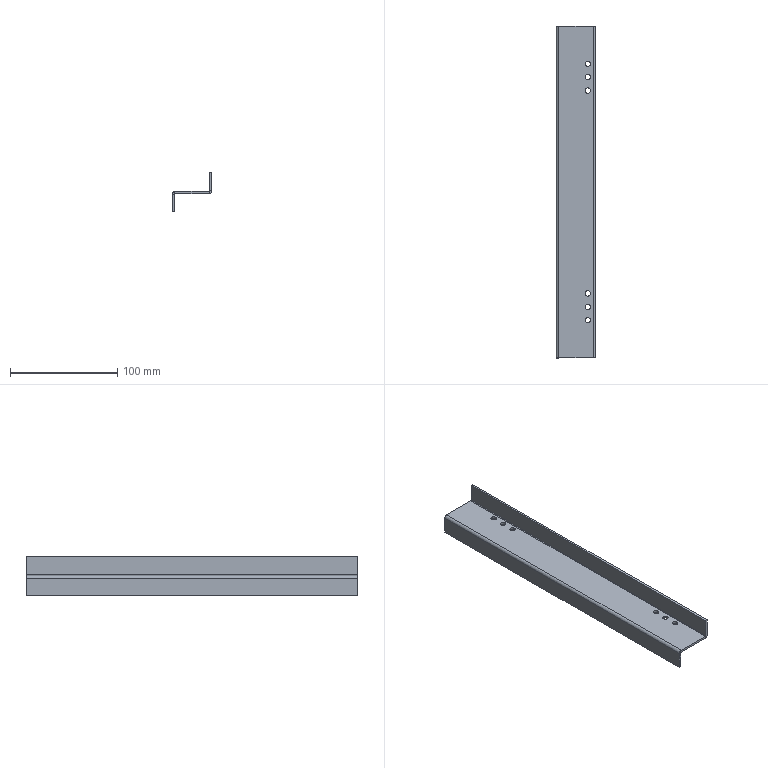Part | SolidWorks | features BaseBody 1 | 1 solid | 34 faces | box 37 x 310 x 36 mm | volume 42986 mm3 | plane 18 | cylinder 16 | commonest cylinder face diameters 5 x14 1 x2
STEP:
#1=CARTESIAN_POINT('',(13.5,119.75,0.));
#2=VERTEX_POINT('',#1);
#3=CARTESIAN_POINT('',(13.5,119.75,-2.));
#4=VERTEX_POINT('',#3);
#5=CARTESIAN_POINT('',(13.5,119.75,0.));
#6=DIRECTION('',(0.,0.,-1.));
#7=VECTOR('',#6,1000.);
#8=LINE('',#5,#7);
#9=EDGE_CURVE('',#2,#4,#8,.T.);
#10=ORIENTED_EDGE('',*,*,#9,.F.);
#11=CARTESIAN_POINT('',(8.5,119.75,0.));
#12=VERTEX_POINT('',#11);
#13=CARTESIAN_POINT('',(11.,119.75,0.));
#14=DIRECTION('',(0.,0.,-1.));
#15=DIRECTION('',(-1.,0.,0.));
#16=AXIS2_PLACEMENT_3D('',#13,#14,#15);
#17=CIRCLE('',#16,2.5);
#18=EDGE_CURVE('',#12,#2,#17,.T.);
#19=ORIENTED_EDGE('',*,*,#18,.F.);
#20=CARTESIAN_POINT('',(8.5,119.75,-2.));
#21=VERTEX_POINT('',#20);
#22=CARTESIAN_POINT('',(8.5,119.75,0.));
#23=DIRECTION('',(0.,0.,-1.));
#24=VECTOR('',#23,1000.);
#25=LINE('',#22,#24);
#26=EDGE_CURVE('',#12,#21,#25,.T.);
#27=ORIENTED_EDGE('',*,*,#26,.T.);
#28=CARTESIAN_POINT('',(11.,119.75,-2.));
#29=DIRECTION('',(0.,0.,-1.));
#30=DIRECTION('',(-1.,0.,0.));
#31=AXIS2_PLACEMENT_3D('',#28,#29,#30);
#32=CIRCLE('',#31,2.5);
#33=EDGE_CURVE('',#21,#4,#32,.T.);
#34=ORIENTED_EDGE('',*,*,#33,.T.);
#35=EDGE_LOOP('',(#10,#19,#27,#34));
#36=FACE_OUTER_BOUND('',#35,.T.);
#37=CARTESIAN_POINT('',(11.,119.75,0.));
#38=DIRECTION('',(0.,0.,-1.));
#39=DIRECTION('',(-1.,0.,0.));
#40=AXIS2_PLACEMENT_3D('',#37,#38,#39);
#41=CYLINDRICAL_SURFACE('',#40,2.5);
#42=ADVANCED_FACE('',(#36),#41,.F.);
#43=CARTESIAN_POINT('',(13.5,94.75,0.));
#44=VERTEX_POINT('',#43);
#45=CARTESIAN_POINT('',(13.5,94.75,-2.));
#46=VERTEX_POINT('',#45);
#47=CARTESIAN_POINT('',(13.5,94.75,0.));
#48=DIRECTION('',(0.,0.,-1.));
#49=VECTOR('',#48,1000.);
#50=LINE('',#47,#49);
#51=EDGE_CURVE('',#44,#46,#50,.T.);
#52=ORIENTED_EDGE('',*,*,#51,.F.);
#53=CARTESIAN_POINT('',(8.5,94.75,0.));
#54=VERTEX_POINT('',#53);
#55=CARTESIAN_POINT('',(11.,94.75,0.));
#56=DIRECTION('',(0.,0.,-1.));
#57=DIRECTION('',(-1.,0.,0.));
#58=AXIS2_PLACEMENT_3D('',#55,#56,#57);
#59=CIRCLE('',#58,2.5);
#60=EDGE_CURVE('',#54,#44,#59,.T.);
#61=ORIENTED_EDGE('',*,*,#60,.F.);
#62=CARTESIAN_POINT('',(8.5,94.75,-2.));
#63=VERTEX_POINT('',#62);
#64=CARTESIAN_POINT('',(8.5,94.75,0.));
#65=DIRECTION('',(0.,0.,-1.));
#66=VECTOR('',#65,1000.);
#67=LINE('',#64,#66);
#68=EDGE_CURVE('',#54,#63,#67,.T.);
#69=ORIENTED_EDGE('',*,*,#68,.T.);
#70=CARTESIAN_POINT('',(11.,94.75,-2.));
#71=DIRECTION('',(0.,0.,-1.));
#72=DIRECTION('',(-1.,0.,0.));
#73=AXIS2_PLACEMENT_3D('',#70,#71,#72);
#74=CIRCLE('',#73,2.5);
#75=EDGE_CURVE('',#63,#46,#74,.T.);
#76=ORIENTED_EDGE('',*,*,#75,.T.);
#77=EDGE_LOOP('',(#52,#61,#69,#76));
#78=FACE_OUTER_BOUND('',#77,.T.);
#79=CARTESIAN_POINT('',(11.,94.75,0.));
#80=DIRECTION('',(0.,0.,-1.));
#81=DIRECTION('',(-1.,0.,0.));
#82=AXIS2_PLACEMENT_3D('',#79,#80,#81);
#83=CYLINDRICAL_SURFACE('',#82,2.5);
#84=ADVANCED_FACE('',(#78),#83,.F.);
#85=CARTESIAN_POINT('',(13.5,-119.75,0.));
#86=VERTEX_POINT('',#85);
#87=CARTESIAN_POINT('',(13.5,-119.75,-2.));
#88=VERTEX_POINT('',#87);
#89=CARTESIAN_POINT('',(13.5,-119.75,0.));
#90=DIRECTION('',(0.,0.,-1.));
#91=VECTOR('',#90,1000.);
#92=LINE('',#89,#91);
#93=EDGE_CURVE('',#86,#88,#92,.T.);
#94=ORIENTED_EDGE('',*,*,#93,.F.);
#95=CARTESIAN_POINT('',(8.5,-119.75,0.));
#96=VERTEX_POINT('',#95);
#97=CARTESIAN_POINT('',(11.,-119.75,0.));
#98=DIRECTION('',(0.,0.,-1.));
#99=DIRECTION('',(1.,0.,0.));
#100=AXIS2_PLACEMENT_3D('',#97,#98,#99);
#101=CIRCLE('',#100,2.5);
#102=EDGE_CURVE('',#96,#86,#101,.T.);
#103=ORIENTED_EDGE('',*,*,#102,.F.);
#104=CARTESIAN_POINT('',(8.5,-119.75,-2.));
#105=VERTEX_POINT('',#104);
#106=CARTESIAN_POINT('',(8.5,-119.75,0.));
#107=DIRECTION('',(0.,0.,-1.));
#108=VECTOR('',#107,1000.);
#109=LINE('',#106,#108);
#110=EDGE_CURVE('',#96,#105,#109,.T.);
#111=ORIENTED_EDGE('',*,*,#110,.T.);
#112=CARTESIAN_POINT('',(11.,-119.75,-2.));
#113=DIRECTION('',(0.,0.,-1.));
#114=DIRECTION('',(1.,0.,0.));
#115=AXIS2_PLACEMENT_3D('',#112,#113,#114);
#116=CIRCLE('',#115,2.5);
#117=EDGE_CURVE('',#105,#88,#116,.T.);
#118=ORIENTED_EDGE('',*,*,#117,.T.);
#119=EDGE_LOOP('',(#94,#103,#111,#118));
#120=FACE_OUTER_BOUND('',#119,.T.);
#121=CARTESIAN_POINT('',(11.,-119.75,0.));
#122=DIRECTION('',(0.,0.,-1.));
#123=DIRECTION('',(-1.,0.,0.));
#124=AXIS2_PLACEMENT_3D('',#121,#122,#123);
#125=CYLINDRICAL_SURFACE('',#124,2.5);
#126=ADVANCED_FACE('',(#120),#125,.F.);
#127=CARTESIAN_POINT('',(13.5,-94.75,0.));
#128=VERTEX_POINT('',#127);
#129=CARTESIAN_POINT('',(13.5,-94.75,-2.));
#130=VERTEX_POINT('',#129);
#131=CARTESIAN_POINT('',(13.5,-94.75,0.));
#132=DIRECTION('',(0.,0.,-1.));
#133=VECTOR('',#132,1000.);
#134=LINE('',#131,#133);
#135=EDGE_CURVE('',#128,#130,#134,.T.);
#136=ORIENTED_EDGE('',*,*,#135,.F.);
#137=CARTESIAN_POINT('',(8.5,-94.75,0.));
#138=VERTEX_POINT('',#137);
#139=CARTESIAN_POINT('',(11.,-94.75,0.));
#140=DIRECTION('',(0.,0.,-1.));
#141=DIRECTION('',(1.,0.,0.));
#142=AXIS2_PLACEMENT_3D('',#139,#140,#141);
#143=CIRCLE('',#142,2.5);
#144=EDGE_CURVE('',#138,#128,#143,.T.);
#145=ORIENTED_EDGE('',*,*,#144,.F.);
#146=CARTESIAN_POINT('',(8.5,-94.75,-2.));
#147=VERTEX_POINT('',#146);
#148=CARTESIAN_POINT('',(8.5,-94.75,0.));
#149=DIRECTION('',(0.,0.,-1.));
#150=VECTOR('',#149,1000.);
#151=LINE('',#148,#150);
#152=EDGE_CURVE('',#138,#147,#151,.T.);
#153=ORIENTED_EDGE('',*,*,#152,.T.);
#154=CARTESIAN_POINT('',(11.,-94.75,-2.));
#155=DIRECTION('',(0.,0.,-1.));
#156=DIRECTION('',(1.,0.,0.));
#157=AXIS2_PLACEMENT_3D('',#154,#155,#156);
#158=CIRCLE('',#157,2.5);
#159=EDGE_CURVE('',#147,#130,#158,.T.);
#160=ORIENTED_EDGE('',*,*,#159,.T.);
#161=EDGE_LOOP('',(#136,#145,#153,#160));
#162=FACE_OUTER_BOUND('',#161,.T.);
#163=CARTESIAN_POINT('',(11.,-94.75,0.));
#164=DIRECTION('',(0.,0.,-1.));
#165=DIRECTION('',(-1.,0.,0.));
#166=AXIS2_PLACEMENT_3D('',#163,#164,#165);
#167=CYLINDRICAL_SURFACE('',#166,2.5);
#168=ADVANCED_FACE('',(#162),#167,.F.);
#169=CARTESIAN_POINT('',(13.5,-107.25,0.));
#170=VERTEX_POINT('',#169);
#171=CARTESIAN_POINT('',(13.5,-107.25,-2.));
#172=VERTEX_POINT('',#171);
#173=CARTESIAN_POINT('',(13.5,-107.25,0.));
#174=DIRECTION('',(0.,0.,-1.));
#175=VECTOR('',#174,1000.);
#176=LINE('',#173,#175);
#177=EDGE_CURVE('',#170,#172,#176,.T.);
#178=ORIENTED_EDGE('',*,*,#177,.F.);
#179=CARTESIAN_POINT('',(8.5,-107.25,0.));
#180=VERTEX_POINT('',#179);
#181=CARTESIAN_POINT('',(11.,-107.25,0.));
#182=DIRECTION('',(0.,0.,-1.));
#183=DIRECTION('',(1.,0.,0.));
#184=AXIS2_PLACEMENT_3D('',#181,#182,#183);
#185=CIRCLE('',#184,2.5);
#186=EDGE_CURVE('',#180,#170,#185,.T.);
#187=ORIENTED_EDGE('',*,*,#186,.F.);
#188=CARTESIAN_POINT('',(8.5,-107.25,-2.));
#189=VERTEX_POINT('',#188);
#190=CARTESIAN_POINT('',(8.5,-107.25,0.));
#191=DIRECTION('',(0.,0.,-1.));
#192=VECTOR('',#191,1000.);
#193=LINE('',#190,#192);
#194=EDGE_CURVE('',#180,#189,#193,.T.);
#195=ORIENTED_EDGE('',*,*,#194,.T.);
#196=CARTESIAN_POINT('',(11.,-107.25,-2.));
#197=DIRECTION('',(0.,0.,-1.));
#198=DIRECTION('',(1.,0.,0.));
#199=AXIS2_PLACEMENT_3D('',#196,#197,#198);
#200=CIRCLE('',#199,2.5);
#201=EDGE_CURVE('',#189,#172,#200,.T.);
#202=ORIENTED_EDGE('',*,*,#201,.T.);
#203=EDGE_LOOP('',(#178,#187,#195,#202));
#204=FACE_OUTER_BOUND('',#203,.T.);
#205=CARTESIAN_POINT('',(11.,-107.25,0.));
#206=DIRECTION('',(0.,0.,-1.));
#207=DIRECTION('',(-1.,0.,0.));
#208=AXIS2_PLACEMENT_3D('',#205,#206,#207);
#209=CYLINDRICAL_SURFACE('',#208,2.5);
#210=ADVANCED_FACE('',(#204),#209,.F.);
#211=CARTESIAN_POINT('',(13.5,107.25,0.));
#212=VERTEX_POINT('',#211);
#213=CARTESIAN_POINT('',(13.5,107.25,-2.));
#214=VERTEX_POINT('',#213);
#215=CARTESIAN_POINT('',(13.5,107.25,0.));
#216=DIRECTION('',(0.,0.,-1.));
#217=VECTOR('',#216,1000.);
#218=LINE('',#215,#217);
#219=EDGE_CURVE('',#212,#214,#218,.T.);
#220=ORIENTED_EDGE('',*,*,#219,.F.);
#221=CARTESIAN_POINT('',(8.5,107.25,0.));
#222=VERTEX_POINT('',#221);
#223=CARTESIAN_POINT('',(11.,107.25,0.));
#224=DIRECTION('',(0.,0.,-1.));
#225=DIRECTION('',(-1.,0.,0.));
#226=AXIS2_PLACEMENT_3D('',#223,#224,#225);
#227=CIRCLE('',#226,2.5);
#228=EDGE_CURVE('',#222,#212,#227,.T.);
#229=ORIENTED_EDGE('',*,*,#228,.F.);
#230=CARTESIAN_POINT('',(8.5,107.25,-2.));
#231=VERTEX_POINT('',#230);
#232=CARTESIAN_POINT('',(8.5,107.25,0.));
#233=DIRECTION('',(0.,0.,-1.));
#234=VECTOR('',#233,1000.);
#235=LINE('',#232,#234);
#236=EDGE_CURVE('',#222,#231,#235,.T.);
#237=ORIENTED_EDGE('',*,*,#236,.T.);
#238=CARTESIAN_POINT('',(11.,107.25,-2.));
#239=DIRECTION('',(0.,0.,-1.));
#240=DIRECTION('',(-1.,0.,0.));
#241=AXIS2_PLACEMENT_3D('',#238,#239,#240);
#242=CIRCLE('',#241,2.5);
#243=EDGE_CURVE('',#231,#214,#242,.T.);
#244=ORIENTED_EDGE('',*,*,#243,.T.);
#245=EDGE_LOOP('',(#220,#229,#237,#244));
#246=FACE_OUTER_BOUND('',#245,.T.);
#247=CARTESIAN_POINT('',(11.,107.25,0.));
#248=DIRECTION('',(0.,0.,-1.));
#249=DIRECTION('',(-1.,0.,0.));
#250=AXIS2_PLACEMENT_3D('',#247,#248,#249);
#251=CYLINDRICAL_SURFACE('',#250,2.5);
#252=ADVANCED_FACE('',(#246),#251,.F.);
#253=CARTESIAN_POINT('',(-16.5,155.,-18.5));
#254=VERTEX_POINT('',#253);
#255=CARTESIAN_POINT('',(-16.5,-155.,-18.5));
#256=VERTEX_POINT('',#255);
#257=CARTESIAN_POINT('',(-16.5,-155.,-18.5));
#258=DIRECTION('',(0.,-1.,0.));
#259=VECTOR('',#258,1000.);
#260=LINE('',#257,#259);
#261=EDGE_CURVE('',#254,#256,#260,.T.);
#262=ORIENTED_EDGE('',*,*,#261,.T.);
#263=CARTESIAN_POINT('',(-18.5,-155.,-18.5));
#264=VERTEX_POINT('',#263);
#265=CARTESIAN_POINT('',(-18.5,-155.,-18.5));
#266=DIRECTION('',(1.,0.,0.));
#267=VECTOR('',#266,1000.);
#268=LINE('',#265,#267);
#269=EDGE_CURVE('',#264,#256,#268,.T.);
#270=ORIENTED_EDGE('',*,*,#269,.F.);
#271=CARTESIAN_POINT('',(-18.5,155.,-18.5));
#272=VERTEX_POINT('',#271);
#273=CARTESIAN_POINT('',(-18.5,0.,-18.5));
#274=DIRECTION('',(0.,-1.,0.));
#275=VECTOR('',#274,1000.);
#276=LINE('',#273,#275);
#277=EDGE_CURVE('',#272,#264,#276,.T.);
#278=ORIENTED_EDGE('',*,*,#277,.F.);
#279=CARTESIAN_POINT('',(-18.5,155.,-18.5));
#280=DIRECTION('',(1.,0.,0.));
#281=VECTOR('',#280,1000.);
#282=LINE('',#279,#281);
#283=EDGE_CURVE('',#272,#254,#282,.T.);
#284=ORIENTED_EDGE('',*,*,#283,.T.);
#285=EDGE_LOOP('',(#262,#270,#278,#284));
#286=FACE_OUTER_BOUND('',#285,.T.);
#287=CARTESIAN_POINT('',(-18.5,-155.,-18.5));
#288=DIRECTION('',(0.,0.,1.));
#289=DIRECTION('',(1.,0.,0.));
#290=AXIS2_PLACEMENT_3D('',#287,#288,#289);
#291=PLANE('',#290);
#292=ADVANCED_FACE('',(#286),#291,.F.);
#293=CARTESIAN_POINT('',(-16.5,155.,-2.5));
#294=VERTEX_POINT('',#293);
#295=CARTESIAN_POINT('',(-16.5,155.,-18.5));
#296=DIRECTION('',(0.,0.,-1.));
#297=VECTOR('',#296,1000.);
#298=LINE('',#295,#297);
#299=EDGE_CURVE('',#294,#254,#298,.T.);
#300=ORIENTED_EDGE('',*,*,#299,.F.);
#301=CARTESIAN_POINT('',(-16.5,-155.,-2.5));
#302=VERTEX_POINT('',#301);
#303=CARTESIAN_POINT('',(-16.5,-155.,-2.5));
#304=DIRECTION('',(0.,1.,0.));
#305=VECTOR('',#304,1000.);
#306=LINE('',#303,#305);
#307=EDGE_CURVE('',#302,#294,#306,.T.);
#308=ORIENTED_EDGE('',*,*,#307,.F.);
#309=CARTESIAN_POINT('',(-16.5,-155.,-2.));
#310=DIRECTION('',(0.,0.,1.));
#311=VECTOR('',#310,1000.);
#312=LINE('',#309,#311);
#313=EDGE_CURVE('',#256,#302,#312,.T.);
#314=ORIENTED_EDGE('',*,*,#313,.F.);
#315=ORIENTED_EDGE('',*,*,#261,.F.);
#316=EDGE_LOOP('',(#300,#308,#314,#315));
#317=FACE_OUTER_BOUND('',#316,.T.);
#318=CARTESIAN_POINT('',(-16.5,0.,0.));
#319=DIRECTION('',(1.,0.,0.));
#320=DIRECTION('',(0.,0.,-1.));
#321=AXIS2_PLACEMENT_3D('',#318,#319,#320);
#322=PLANE('',#321);
#323=ADVANCED_FACE('',(#317),#322,.T.);
#324=CARTESIAN_POINT('',(-18.5,155.,-2.5));
#325=VERTEX_POINT('',#324);
#326=CARTESIAN_POINT('',(-18.5,-155.,-2.5));
#327=VERTEX_POINT('',#326);
#328=CARTESIAN_POINT('',(-18.5,-155.,-2.5));
#329=DIRECTION('',(0.,-1.,0.));
#330=VECTOR('',#329,1000.);
#331=LINE('',#328,#330);
#332=EDGE_CURVE('',#325,#327,#331,.T.);
#333=ORIENTED_EDGE('',*,*,#332,.F.);
#334=CARTESIAN_POINT('',(-18.5,155.,0.));
#335=DIRECTION('',(0.,0.,-1.));
#336=VECTOR('',#335,1000.);
#337=LINE('',#334,#336);
#338=EDGE_CURVE('',#325,#272,#337,.T.);
#339=ORIENTED_EDGE('',*,*,#338,.T.);
#340=ORIENTED_EDGE('',*,*,#277,.T.);
#341=CARTESIAN_POINT('',(-18.5,-155.,0.));
#342=DIRECTION('',(0.,0.,1.));
#343=VECTOR('',#342,1000.);
#344=LINE('',#341,#343);
#345=EDGE_CURVE('',#264,#327,#344,.T.);
#346=ORIENTED_EDGE('',*,*,#345,.T.);
#347=EDGE_LOOP('',(#333,#339,#340,#346));
#348=FACE_OUTER_BOUND('',#347,.T.);
#349=CARTESIAN_POINT('',(-18.5,0.,0.));
#350=DIRECTION('',(1.,0.,0.));
#351=DIRECTION('',(0.,0.,-1.));
#352=AXIS2_PLACEMENT_3D('',#349,#350,#351);
#353=PLANE('',#352);
#354=ADVANCED_FACE('',(#348),#353,.F.);
#355=CARTESIAN_POINT('',(-18.5,-155.,-2.5));
#356=DIRECTION('',(-1.,0.,0.));
#357=VECTOR('',#356,1000.);
#358=LINE('',#355,#357);
#359=EDGE_CURVE('',#302,#327,#358,.T.);
#360=ORIENTED_EDGE('',*,*,#359,.T.);
#361=ORIENTED_EDGE('',*,*,#345,.F.);
#362=ORIENTED_EDGE('',*,*,#269,.T.);
#363=ORIENTED_EDGE('',*,*,#313,.T.);
#364=EDGE_LOOP('',(#360,#361,#362,#363));
#365=FACE_OUTER_BOUND('',#364,.T.);
#366=CARTESIAN_POINT('',(-18.5,-155.,-2.));
#367=DIRECTION('',(0.,1.,0.));
#368=DIRECTION('',(1.,0.,0.));
#369=AXIS2_PLACEMENT_3D('',#366,#367,#368);
#370=PLANE('',#369);
#371=ADVANCED_FACE('',(#365),#370,.F.);
#372=CARTESIAN_POINT('',(-16.5,155.,-2.5));
#373=DIRECTION('',(-1.,0.,0.));
#374=VECTOR('',#373,1000.);
#375=LINE('',#372,#374);
#376=EDGE_CURVE('',#294,#325,#375,.T.);
#377=ORIENTED_EDGE('',*,*,#376,.F.);
#378=ORIENTED_EDGE('',*,*,#299,.T.);
#379=ORIENTED_EDGE('',*,*,#283,.F.);
#380=ORIENTED_EDGE('',*,*,#338,.F.);
#381=EDGE_LOOP('',(#377,#378,#379,#380));
#382=FACE_OUTER_BOUND('',#381,.T.);
#383=CARTESIAN_POINT('',(-18.5,155.,-18.5));
#384=DIRECTION('',(0.,-1.,0.));
#385=DIRECTION('',(0.,0.,-1.));
#386=AXIS2_PLACEMENT_3D('',#383,#384,#385);
#387=PLANE('',#386);
#388=ADVANCED_FACE('',(#382),#387,.F.);
#389=CARTESIAN_POINT('',(-16.,155.,-2.));
#390=VERTEX_POINT('',#389);
#391=CARTESIAN_POINT('',(-16.,-155.,-2.));
#392=VERTEX_POINT('',#391);
#393=CARTESIAN_POINT('',(-16.,155.,-2.));
#394=DIRECTION('',(0.,-1.,0.));
#395=VECTOR('',#394,1000.);
#396=LINE('',#393,#395);
#397=EDGE_CURVE('',#390,#392,#396,.T.);
#398=ORIENTED_EDGE('',*,*,#397,.T.);
#399=CARTESIAN_POINT('',(-16.,-155.,-2.5));
#400=DIRECTION('',(0.,-1.,0.));
#401=DIRECTION('',(0.,0.,1.));
#402=AXIS2_PLACEMENT_3D('',#399,#400,#401);
#403=CIRCLE('',#402,0.5);
#404=EDGE_CURVE('',#392,#302,#403,.T.);
#405=ORIENTED_EDGE('',*,*,#404,.T.);
#406=ORIENTED_EDGE('',*,*,#307,.T.);
#407=CARTESIAN_POINT('',(-16.,155.,-2.5));
#408=DIRECTION('',(0.,1.,0.));
#409=DIRECTION('',(0.,0.,1.));
#410=AXIS2_PLACEMENT_3D('',#407,#408,#409);
#411=CIRCLE('',#410,0.5);
#412=EDGE_CURVE('',#294,#390,#411,.T.);
#413=ORIENTED_EDGE('',*,*,#412,.T.);
#414=EDGE_LOOP('',(#398,#405,#406,#413));
#415=FACE_OUTER_BOUND('',#414,.T.);
#416=CARTESIAN_POINT('',(-16.,155.,-2.5));
#417=DIRECTION('',(0.,1.,0.));
#418=DIRECTION('',(-1.,0.,0.));
#419=AXIS2_PLACEMENT_3D('',#416,#417,#418);
#420=CYLINDRICAL_SURFACE('',#419,0.5);
#421=ADVANCED_FACE('',(#415),#420,.F.);
#422=CARTESIAN_POINT('',(-16.,155.,0.));
#423=VERTEX_POINT('',#422);
#424=CARTESIAN_POINT('',(-16.,-155.,0.));
#425=VERTEX_POINT('',#424);
#426=CARTESIAN_POINT('',(-16.,155.,0.));
#427=DIRECTION('',(0.,-1.,0.));
#428=VECTOR('',#427,1000.);
#429=LINE('',#426,#428);
#430=EDGE_CURVE('',#423,#425,#429,.T.);
#431=ORIENTED_EDGE('',*,*,#430,.F.);
#432=CARTESIAN_POINT('',(-16.,155.,-2.5));
#433=DIRECTION('',(0.,1.,0.));
#434=DIRECTION('',(0.,0.,1.));
#435=AXIS2_PLACEMENT_3D('',#432,#433,#434);
#436=CIRCLE('',#435,2.5);
#437=EDGE_CURVE('',#325,#423,#436,.T.);
#438=ORIENTED_EDGE('',*,*,#437,.F.);
#439=ORIENTED_EDGE('',*,*,#332,.T.);
#440=CARTESIAN_POINT('',(-16.,-155.,-2.5));
#441=DIRECTION('',(0.,-1.,0.));
#442=DIRECTION('',(0.,0.,1.));
#443=AXIS2_PLACEMENT_3D('',#440,#441,#442);
#444=CIRCLE('',#443,2.5);
#445=EDGE_CURVE('',#425,#327,#444,.T.);
#446=ORIENTED_EDGE('',*,*,#445,.F.);
#447=EDGE_LOOP('',(#431,#438,#439,#446));
#448=FACE_OUTER_BOUND('',#447,.T.);
#449=CARTESIAN_POINT('',(-16.,155.,-2.5));
#450=DIRECTION('',(0.,1.,0.));
#451=DIRECTION('',(-1.,0.,0.));
#452=AXIS2_PLACEMENT_3D('',#449,#450,#451);
#453=CYLINDRICAL_SURFACE('',#452,2.5);
#454=ADVANCED_FACE('',(#448),#453,.T.);
#455=ORIENTED_EDGE('',*,*,#412,.F.);
#456=ORIENTED_EDGE('',*,*,#376,.T.);
#457=ORIENTED_EDGE('',*,*,#437,.T.);
#458=CARTESIAN_POINT('',(-16.,155.,-2.));
#459=DIRECTION('',(0.,0.,1.));
#460=VECTOR('',#459,1000.);
#461=LINE('',#458,#460);
#462=EDGE_CURVE('',#390,#423,#461,.T.);
#463=ORIENTED_EDGE('',*,*,#462,.F.);
#464=EDGE_LOOP('',(#455,#456,#457,#463));
#465=FACE_OUTER_BOUND('',#464,.T.);
#466=CARTESIAN_POINT('',(-16.,155.,-2.5));
#467=DIRECTION('',(0.,-1.,0.));
#468=DIRECTION('',(0.,0.,-1.));
#469=AXIS2_PLACEMENT_3D('',#466,#467,#468);
#470=PLANE('',#469);
#471=ADVANCED_FACE('',(#465),#470,.F.);
#472=ORIENTED_EDGE('',*,*,#359,.F.);
#473=ORIENTED_EDGE('',*,*,#404,.F.);
#474=CARTESIAN_POINT('',(-16.,-155.,-2.));
#475=DIRECTION('',(0.,0.,1.));
#476=VECTOR('',#475,1000.);
#477=LINE('',#474,#476);
#478=EDGE_CURVE('',#392,#425,#477,.T.);
#479=ORIENTED_EDGE('',*,*,#478,.T.);
#480=ORIENTED_EDGE('',*,*,#445,.T.);
#481=EDGE_LOOP('',(#472,#473,#479,#480));
#482=FACE_OUTER_BOUND('',#481,.T.);
#483=CARTESIAN_POINT('',(-16.,-155.,-2.5));
#484=DIRECTION('',(0.,-1.,0.));
#485=DIRECTION('',(0.,0.,-1.));
#486=AXIS2_PLACEMENT_3D('',#483,#484,#485);
#487=PLANE('',#486);
#488=ADVANCED_FACE('',(#482),#487,.T.);
#489=CARTESIAN_POINT('',(16.5,155.,17.5));
#490=VERTEX_POINT('',#489);
#491=CARTESIAN_POINT('',(16.5,-155.,17.5));
#492=VERTEX_POINT('',#491);
#493=CARTESIAN_POINT('',(16.5,-155.,17.5));
#494=DIRECTION('',(0.,-1.,0.));
#495=VECTOR('',#494,1000.);
#496=LINE('',#493,#495);
#497=EDGE_CURVE('',#490,#492,#496,.T.);
#498=ORIENTED_EDGE('',*,*,#497,.T.);
#499=CARTESIAN_POINT('',(18.5,-155.,17.5));
#500=VERTEX_POINT('',#499);
#501=CARTESIAN_POINT('',(18.5,-155.,17.5));
#502=DIRECTION('',(-1.,0.,0.));
#503=VECTOR('',#502,1000.);
#504=LINE('',#501,#503);
#505=EDGE_CURVE('',#500,#492,#504,.T.);
#506=ORIENTED_EDGE('',*,*,#505,.F.);
#507=CARTESIAN_POINT('',(18.5,155.,17.5));
#508=VERTEX_POINT('',#507);
#509=CARTESIAN_POINT('',(18.5,0.,17.5));
#510=DIRECTION('',(0.,-1.,0.));
#511=VECTOR('',#510,1000.);
#512=LINE('',#509,#511);
#513=EDGE_CURVE('',#508,#500,#512,.T.);
#514=ORIENTED_EDGE('',*,*,#513,.F.);
#515=CARTESIAN_POINT('',(18.5,155.,17.5));
#516=DIRECTION('',(-1.,0.,0.));
#517=VECTOR('',#516,1000.);
#518=LINE('',#515,#517);
#519=EDGE_CURVE('',#508,#490,#518,.T.);
#520=ORIENTED_EDGE('',*,*,#519,.T.);
#521=EDGE_LOOP('',(#498,#506,#514,#520));
#522=FACE_OUTER_BOUND('',#521,.T.);
#523=CARTESIAN_POINT('',(18.5,-155.,17.5));
#524=DIRECTION('',(0.,0.,-1.));
#525=DIRECTION('',(-1.,0.,0.));
#526=AXIS2_PLACEMENT_3D('',#523,#524,#525);
#527=PLANE('',#526);
#528=ADVANCED_FACE('',(#522),#527,.F.);
#529=CARTESIAN_POINT('',(16.5,155.,0.5));
#530=VERTEX_POINT('',#529);
#531=CARTESIAN_POINT('',(16.5,155.,17.5));
#532=DIRECTION('',(0.,0.,1.));
#533=VECTOR('',#532,1000.);
#534=LINE('',#531,#533);
#535=EDGE_CURVE('',#530,#490,#534,.T.);
#536=ORIENTED_EDGE('',*,*,#535,.F.);
#537=CARTESIAN_POINT('',(16.5,-155.,0.5));
#538=VERTEX_POINT('',#537);
#539=CARTESIAN_POINT('',(16.5,-155.,0.5));
#540=DIRECTION('',(0.,1.,0.));
#541=VECTOR('',#540,1000.);
#542=LINE('',#539,#541);
#543=EDGE_CURVE('',#538,#530,#542,.T.);
#544=ORIENTED_EDGE('',*,*,#543,.F.);
#545=CARTESIAN_POINT('',(16.5,-155.,0.));
#546=DIRECTION('',(0.,0.,-1.));
#547=VECTOR('',#546,1000.);
#548=LINE('',#545,#547);
#549=EDGE_CURVE('',#492,#538,#548,.T.);
#550=ORIENTED_EDGE('',*,*,#549,.F.);
#551=ORIENTED_EDGE('',*,*,#497,.F.);
#552=EDGE_LOOP('',(#536,#544,#550,#551));
#553=FACE_OUTER_BOUND('',#552,.T.);
#554=CARTESIAN_POINT('',(16.5,0.,0.));
#555=DIRECTION('',(-1.,0.,0.));
#556=DIRECTION('',(0.,1.,0.));
#557=AXIS2_PLACEMENT_3D('',#554,#555,#556);
#558=PLANE('',#557);
#559=ADVANCED_FACE('',(#553),#558,.T.);
#560=CARTESIAN_POINT('',(18.5,155.,0.5));
#561=VERTEX_POINT('',#560);
#562=CARTESIAN_POINT('',(18.5,-155.,0.5));
#563=VERTEX_POINT('',#562);
#564=CARTESIAN_POINT('',(18.5,-155.,0.5));
#565=DIRECTION('',(0.,-1.,0.));
#566=VECTOR('',#565,1000.);
#567=LINE('',#564,#566);
#568=EDGE_CURVE('',#561,#563,#567,.T.);
#569=ORIENTED_EDGE('',*,*,#568,.F.);
#570=CARTESIAN_POINT('',(18.5,155.,0.));
#571=DIRECTION('',(0.,0.,1.));
#572=VECTOR('',#571,1000.);
#573=LINE('',#570,#572);
#574=EDGE_CURVE('',#561,#508,#573,.T.);
#575=ORIENTED_EDGE('',*,*,#574,.T.);
#576=ORIENTED_EDGE('',*,*,#513,.T.);
#577=CARTESIAN_POINT('',(18.5,-155.,0.));
#578=DIRECTION('',(0.,0.,-1.));
#579=VECTOR('',#578,1000.);
#580=LINE('',#577,#579);
#581=EDGE_CURVE('',#500,#563,#580,.T.);
#582=ORIENTED_EDGE('',*,*,#581,.T.);
#583=EDGE_LOOP('',(#569,#575,#576,#582));
#584=FACE_OUTER_BOUND('',#583,.T.);
#585=CARTESIAN_POINT('',(18.5,0.,0.));
#586=DIRECTION('',(-1.,0.,0.));
#587=DIRECTION('',(0.,1.,0.));
#588=AXIS2_PLACEMENT_3D('',#585,#586,#587);
#589=PLANE('',#588);
#590=ADVANCED_FACE('',(#584),#589,.F.);
#591=CARTESIAN_POINT('',(16.5,155.,0.5));
#592=DIRECTION('',(1.,0.,0.));
#593=VECTOR('',#592,1000.);
#594=LINE('',#591,#593);
#595=EDGE_CURVE('',#530,#561,#594,.T.);
#596=ORIENTED_EDGE('',*,*,#595,.F.);
#597=ORIENTED_EDGE('',*,*,#535,.T.);
#598=ORIENTED_EDGE('',*,*,#519,.F.);
#599=ORIENTED_EDGE('',*,*,#574,.F.);
#600=EDGE_LOOP('',(#596,#597,#598,#599));
#601=FACE_OUTER_BOUND('',#600,.T.);
#602=CARTESIAN_POINT('',(18.5,155.,17.5));
#603=DIRECTION('',(0.,-1.,0.));
#604=DIRECTION('',(0.,0.,-1.));
#605=AXIS2_PLACEMENT_3D('',#602,#603,#604);
#606=PLANE('',#605);
#607=ADVANCED_FACE('',(#601),#606,.F.);
#608=CARTESIAN_POINT('',(18.5,-155.,0.5));
#609=DIRECTION('',(1.,0.,0.));
#610=VECTOR('',#609,1000.);
#611=LINE('',#608,#610);
#612=EDGE_CURVE('',#538,#563,#611,.T.);
#613=ORIENTED_EDGE('',*,*,#612,.T.);
#614=ORIENTED_EDGE('',*,*,#581,.F.);
#615=ORIENTED_EDGE('',*,*,#505,.T.);
#616=ORIENTED_EDGE('',*,*,#549,.T.);
#617=EDGE_LOOP('',(#613,#614,#615,#616));
#618=FACE_OUTER_BOUND('',#617,.T.);
#619=CARTESIAN_POINT('',(18.5,-155.,0.));
#620=DIRECTION('',(0.,1.,0.));
#621=DIRECTION('',(1.,0.,0.));
#622=AXIS2_PLACEMENT_3D('',#619,#620,#621);
#623=PLANE('',#622);
#624=ADVANCED_FACE('',(#618),#623,.F.);
#625=CARTESIAN_POINT('',(16.,155.,0.));
#626=VERTEX_POINT('',#625);
#627=CARTESIAN_POINT('',(16.,-155.,0.));
#628=VERTEX_POINT('',#627);
#629=CARTESIAN_POINT('',(16.,155.,0.));
#630=DIRECTION('',(0.,-1.,0.));
#631=VECTOR('',#630,1000.);
#632=LINE('',#629,#631);
#633=EDGE_CURVE('',#626,#628,#632,.T.);
#634=ORIENTED_EDGE('',*,*,#633,.T.);
#635=CARTESIAN_POINT('',(16.,-155.,0.5));
#636=DIRECTION('',(0.,-1.,0.));
#637=DIRECTION('',(0.,0.,1.));
#638=AXIS2_PLACEMENT_3D('',#635,#636,#637);
#639=CIRCLE('',#638,0.5);
#640=EDGE_CURVE('',#628,#538,#639,.T.);
#641=ORIENTED_EDGE('',*,*,#640,.T.);
#642=ORIENTED_EDGE('',*,*,#543,.T.);
#643=CARTESIAN_POINT('',(16.,155.,0.5));
#644=DIRECTION('',(0.,1.,0.));
#645=DIRECTION('',(0.,0.,1.));
#646=AXIS2_PLACEMENT_3D('',#643,#644,#645);
#647=CIRCLE('',#646,0.5);
#648=EDGE_CURVE('',#530,#626,#647,.T.);
#649=ORIENTED_EDGE('',*,*,#648,.T.);
#650=EDGE_LOOP('',(#634,#641,#642,#649));
#651=FACE_OUTER_BOUND('',#650,.T.);
#652=CARTESIAN_POINT('',(16.,155.,0.5));
#653=DIRECTION('',(0.,1.,0.));
#654=DIRECTION('',(1.,0.,0.));
#655=AXIS2_PLACEMENT_3D('',#652,#653,#654);
#656=CYLINDRICAL_SURFACE('',#655,0.5);
#657=ADVANCED_FACE('',(#651),#656,.F.);
#658=CARTESIAN_POINT('',(16.,155.,-2.));
#659=VERTEX_POINT('',#658);
#660=CARTESIAN_POINT('',(16.,-155.,-2.));
#661=VERTEX_POINT('',#660);
#662=CARTESIAN_POINT('',(16.,155.,-2.));
#663=DIRECTION('',(0.,-1.,0.));
#664=VECTOR('',#663,1000.);
#665=LINE('',#662,#664);
#666=EDGE_CURVE('',#659,#661,#665,.T.);
#667=ORIENTED_EDGE('',*,*,#666,.F.);
#668=CARTESIAN_POINT('',(16.,155.,0.5));
#669=DIRECTION('',(0.,1.,0.));
#670=DIRECTION('',(0.,0.,1.));
#671=AXIS2_PLACEMENT_3D('',#668,#669,#670);
#672=CIRCLE('',#671,2.5);
#673=EDGE_CURVE('',#561,#659,#672,.T.);
#674=ORIENTED_EDGE('',*,*,#673,.F.);
#675=ORIENTED_EDGE('',*,*,#568,.T.);
#676=CARTESIAN_POINT('',(16.,-155.,0.5));
#677=DIRECTION('',(0.,-1.,0.));
#678=DIRECTION('',(0.,0.,1.));
#679=AXIS2_PLACEMENT_3D('',#676,#677,#678);
#680=CIRCLE('',#679,2.5);
#681=EDGE_CURVE('',#661,#563,#680,.T.);
#682=ORIENTED_EDGE('',*,*,#681,.F.);
#683=EDGE_LOOP('',(#667,#674,#675,#682));
#684=FACE_OUTER_BOUND('',#683,.T.);
#685=CARTESIAN_POINT('',(16.,155.,0.5));
#686=DIRECTION('',(0.,1.,0.));
#687=DIRECTION('',(1.,0.,0.));
#688=AXIS2_PLACEMENT_3D('',#685,#686,#687);
#689=CYLINDRICAL_SURFACE('',#688,2.5);
#690=ADVANCED_FACE('',(#684),#689,.T.);
#691=ORIENTED_EDGE('',*,*,#648,.F.);
#692=ORIENTED_EDGE('',*,*,#595,.T.);
#693=ORIENTED_EDGE('',*,*,#673,.T.);
#694=CARTESIAN_POINT('',(16.,155.,0.));
#695=DIRECTION('',(0.,0.,-1.));
#696=VECTOR('',#695,1000.);
#697=LINE('',#694,#696);
#698=EDGE_CURVE('',#626,#659,#697,.T.);
#699=ORIENTED_EDGE('',*,*,#698,.F.);
#700=EDGE_LOOP('',(#691,#692,#693,#699));
#701=FACE_OUTER_BOUND('',#700,.T.);
#702=CARTESIAN_POINT('',(16.,155.,0.5));
#703=DIRECTION('',(0.,-1.,0.));
#704=DIRECTION('',(0.,0.,-1.));
#705=AXIS2_PLACEMENT_3D('',#702,#703,#704);
#706=PLANE('',#705);
#707=ADVANCED_FACE('',(#701),#706,.F.);
#708=ORIENTED_EDGE('',*,*,#612,.F.);
#709=ORIENTED_EDGE('',*,*,#640,.F.);
#710=CARTESIAN_POINT('',(16.,-155.,0.));
#711=DIRECTION('',(0.,0.,-1.));
#712=VECTOR('',#711,1000.);
#713=LINE('',#710,#712);
#714=EDGE_CURVE('',#628,#661,#713,.T.);
#715=ORIENTED_EDGE('',*,*,#714,.T.);
#716=ORIENTED_EDGE('',*,*,#681,.T.);
#717=EDGE_LOOP('',(#708,#709,#715,#716));
#718=FACE_OUTER_BOUND('',#717,.T.);
#719=CARTESIAN_POINT('',(16.,-155.,0.5));
#720=DIRECTION('',(0.,-1.,0.));
#721=DIRECTION('',(0.,0.,-1.));
#722=AXIS2_PLACEMENT_3D('',#719,#720,#721);
#723=PLANE('',#722);
#724=ADVANCED_FACE('',(#718),#723,.T.);
#725=ORIENTED_EDGE('',*,*,#478,.F.);
#726=CARTESIAN_POINT('',(18.5,-155.,-2.));
#727=DIRECTION('',(1.,0.,0.));
#728=VECTOR('',#727,1000.);
#729=LINE('',#726,#728);
#730=EDGE_CURVE('',#392,#661,#729,.T.);
#731=ORIENTED_EDGE('',*,*,#730,.T.);
#732=ORIENTED_EDGE('',*,*,#714,.F.);
#733=CARTESIAN_POINT('',(18.5,-155.,0.));
#734=DIRECTION('',(1.,0.,0.));
#735=VECTOR('',#734,1000.);
#736=LINE('',#733,#735);
#737=EDGE_CURVE('',#425,#628,#736,.T.);
#738=ORIENTED_EDGE('',*,*,#737,.F.);
#739=EDGE_LOOP('',(#725,#731,#732,#738));
#740=FACE_OUTER_BOUND('',#739,.T.);
#741=CARTESIAN_POINT('',(18.5,-155.,-2.));
#742=DIRECTION('',(0.,-1.,0.));
#743=DIRECTION('',(0.,0.,-1.));
#744=AXIS2_PLACEMENT_3D('',#741,#742,#743);
#745=PLANE('',#744);
#746=ADVANCED_FACE('',(#740),#745,.T.);
#747=ORIENTED_EDGE('',*,*,#228,.T.);
#748=CARTESIAN_POINT('',(11.,107.25,0.));
#749=DIRECTION('',(0.,0.,-1.));
#750=DIRECTION('',(-1.,0.,0.));
#751=AXIS2_PLACEMENT_3D('',#748,#749,#750);
#752=CIRCLE('',#751,2.5);
#753=EDGE_CURVE('',#212,#222,#752,.T.);
#754=ORIENTED_EDGE('',*,*,#753,.T.);
#755=EDGE_LOOP('',(#747,#754));
#756=FACE_BOUND('',#755,.T.);
#757=ORIENTED_EDGE('',*,*,#186,.T.);
#758=CARTESIAN_POINT('',(11.,-107.25,0.));
#759=DIRECTION('',(0.,0.,-1.));
#760=DIRECTION('',(1.,0.,0.));
#761=AXIS2_PLACEMENT_3D('',#758,#759,#760);
#762=CIRCLE('',#761,2.5);
#763=EDGE_CURVE('',#170,#180,#762,.T.);
#764=ORIENTED_EDGE('',*,*,#763,.T.);
#765=EDGE_LOOP('',(#757,#764));
#766=FACE_BOUND('',#765,.T.);
#767=ORIENTED_EDGE('',*,*,#144,.T.);
#768=CARTESIAN_POINT('',(11.,-94.75,0.));
#769=DIRECTION('',(0.,0.,-1.));
#770=DIRECTION('',(1.,0.,0.));
#771=AXIS2_PLACEMENT_3D('',#768,#769,#770);
#772=CIRCLE('',#771,2.5);
#773=EDGE_CURVE('',#128,#138,#772,.T.);
#774=ORIENTED_EDGE('',*,*,#773,.T.);
#775=EDGE_LOOP('',(#767,#774));
#776=FACE_BOUND('',#775,.T.);
#777=ORIENTED_EDGE('',*,*,#102,.T.);
#778=CARTESIAN_POINT('',(11.,-119.75,0.));
#779=DIRECTION('',(0.,0.,-1.));
#780=DIRECTION('',(1.,0.,0.));
#781=AXIS2_PLACEMENT_3D('',#778,#779,#780);
#782=CIRCLE('',#781,2.5);
#783=EDGE_CURVE('',#86,#96,#782,.T.);
#784=ORIENTED_EDGE('',*,*,#783,.T.);
#785=EDGE_LOOP('',(#777,#784));
#786=FACE_BOUND('',#785,.T.);
#787=ORIENTED_EDGE('',*,*,#60,.T.);
#788=CARTESIAN_POINT('',(11.,94.75,0.));
#789=DIRECTION('',(0.,0.,-1.));
#790=DIRECTION('',(-1.,0.,0.));
#791=AXIS2_PLACEMENT_3D('',#788,#789,#790);
#792=CIRCLE('',#791,2.5);
#793=EDGE_CURVE('',#44,#54,#792,.T.);
#794=ORIENTED_EDGE('',*,*,#793,.T.);
#795=EDGE_LOOP('',(#787,#794));
#796=FACE_BOUND('',#795,.T.);
#797=ORIENTED_EDGE('',*,*,#18,.T.);
#798=CARTESIAN_POINT('',(11.,119.75,0.));
#799=DIRECTION('',(0.,0.,-1.));
#800=DIRECTION('',(-1.,0.,0.));
#801=AXIS2_PLACEMENT_3D('',#798,#799,#800);
#802=CIRCLE('',#801,2.5);
#803=EDGE_CURVE('',#2,#12,#802,.T.);
#804=ORIENTED_EDGE('',*,*,#803,.T.);
#805=EDGE_LOOP('',(#797,#804));
#806=FACE_BOUND('',#805,.T.);
#807=ORIENTED_EDGE('',*,*,#430,.T.);
#808=ORIENTED_EDGE('',*,*,#737,.T.);
#809=ORIENTED_EDGE('',*,*,#633,.F.);
#810=CARTESIAN_POINT('',(18.5,155.,0.));
#811=DIRECTION('',(-1.,0.,0.));
#812=VECTOR('',#811,1000.);
#813=LINE('',#810,#812);
#814=EDGE_CURVE('',#626,#423,#813,.T.);
#815=ORIENTED_EDGE('',*,*,#814,.T.);
#816=EDGE_LOOP('',(#807,#808,#809,#815));
#817=FACE_OUTER_BOUND('',#816,.T.);
#818=CARTESIAN_POINT('',(0.,0.,0.));
#819=DIRECTION('',(0.,0.,-1.));
#820=DIRECTION('',(0.,-1.,0.));
#821=AXIS2_PLACEMENT_3D('',#818,#819,#820);
#822=PLANE('',#821);
#823=ADVANCED_FACE('',(#756,#766,#776,#786,#796,#806,#817),#822,.F.);
#824=ORIENTED_EDGE('',*,*,#243,.F.);
#825=CARTESIAN_POINT('',(11.,107.25,-2.));
#826=DIRECTION('',(0.,0.,-1.));
#827=DIRECTION('',(-1.,0.,0.));
#828=AXIS2_PLACEMENT_3D('',#825,#826,#827);
#829=CIRCLE('',#828,2.5);
#830=EDGE_CURVE('',#214,#231,#829,.T.);
#831=ORIENTED_EDGE('',*,*,#830,.F.);
#832=EDGE_LOOP('',(#824,#831));
#833=FACE_BOUND('',#832,.T.);
#834=ORIENTED_EDGE('',*,*,#201,.F.);
#835=CARTESIAN_POINT('',(11.,-107.25,-2.));
#836=DIRECTION('',(0.,0.,-1.));
#837=DIRECTION('',(1.,0.,0.));
#838=AXIS2_PLACEMENT_3D('',#835,#836,#837);
#839=CIRCLE('',#838,2.5);
#840=EDGE_CURVE('',#172,#189,#839,.T.);
#841=ORIENTED_EDGE('',*,*,#840,.F.);
#842=EDGE_LOOP('',(#834,#841));
#843=FACE_BOUND('',#842,.T.);
#844=ORIENTED_EDGE('',*,*,#159,.F.);
#845=CARTESIAN_POINT('',(11.,-94.75,-2.));
#846=DIRECTION('',(0.,0.,-1.));
#847=DIRECTION('',(1.,0.,0.));
#848=AXIS2_PLACEMENT_3D('',#845,#846,#847);
#849=CIRCLE('',#848,2.5);
#850=EDGE_CURVE('',#130,#147,#849,.T.);
#851=ORIENTED_EDGE('',*,*,#850,.F.);
#852=EDGE_LOOP('',(#844,#851));
#853=FACE_BOUND('',#852,.T.);
#854=ORIENTED_EDGE('',*,*,#117,.F.);
#855=CARTESIAN_POINT('',(11.,-119.75,-2.));
#856=DIRECTION('',(0.,0.,-1.));
#857=DIRECTION('',(1.,0.,0.));
#858=AXIS2_PLACEMENT_3D('',#855,#856,#857);
#859=CIRCLE('',#858,2.5);
#860=EDGE_CURVE('',#88,#105,#859,.T.);
#861=ORIENTED_EDGE('',*,*,#860,.F.);
#862=EDGE_LOOP('',(#854,#861));
#863=FACE_BOUND('',#862,.T.);
#864=ORIENTED_EDGE('',*,*,#75,.F.);
#865=CARTESIAN_POINT('',(11.,94.75,-2.));
#866=DIRECTION('',(0.,0.,-1.));
#867=DIRECTION('',(-1.,0.,0.));
#868=AXIS2_PLACEMENT_3D('',#865,#866,#867);
#869=CIRCLE('',#868,2.5);
#870=EDGE_CURVE('',#46,#63,#869,.T.);
#871=ORIENTED_EDGE('',*,*,#870,.F.);
#872=EDGE_LOOP('',(#864,#871));
#873=FACE_BOUND('',#872,.T.);
#874=ORIENTED_EDGE('',*,*,#33,.F.);
#875=CARTESIAN_POINT('',(11.,119.75,-2.));
#876=DIRECTION('',(0.,0.,-1.));
#877=DIRECTION('',(-1.,0.,0.));
#878=AXIS2_PLACEMENT_3D('',#875,#876,#877);
#879=CIRCLE('',#878,2.5);
#880=EDGE_CURVE('',#4,#21,#879,.T.);
#881=ORIENTED_EDGE('',*,*,#880,.F.);
#882=EDGE_LOOP('',(#874,#881));
#883=FACE_BOUND('',#882,.T.);
#884=ORIENTED_EDGE('',*,*,#730,.F.);
#885=ORIENTED_EDGE('',*,*,#397,.F.);
#886=CARTESIAN_POINT('',(18.5,155.,-2.));
#887=DIRECTION('',(-1.,0.,0.));
#888=VECTOR('',#887,1000.);
#889=LINE('',#886,#888);
#890=EDGE_CURVE('',#659,#390,#889,.T.);
#891=ORIENTED_EDGE('',*,*,#890,.F.);
#892=ORIENTED_EDGE('',*,*,#666,.T.);
#893=EDGE_LOOP('',(#884,#885,#891,#892));
#894=FACE_OUTER_BOUND('',#893,.T.);
#895=CARTESIAN_POINT('',(0.,0.,-2.));
#896=DIRECTION('',(0.,0.,-1.));
#897=DIRECTION('',(0.,-1.,0.));
#898=AXIS2_PLACEMENT_3D('',#895,#896,#897);
#899=PLANE('',#898);
#900=ADVANCED_FACE('',(#833,#843,#853,#863,#873,#883,#894),#899,.T.);
#901=ORIENTED_EDGE('',*,*,#890,.T.);
#902=ORIENTED_EDGE('',*,*,#462,.T.);
#903=ORIENTED_EDGE('',*,*,#814,.F.);
#904=ORIENTED_EDGE('',*,*,#698,.T.);
#905=EDGE_LOOP('',(#901,#902,#903,#904));
#906=FACE_OUTER_BOUND('',#905,.T.);
#907=CARTESIAN_POINT('',(18.5,155.,-2.));
#908=DIRECTION('',(0.,1.,0.));
#909=DIRECTION('',(1.,0.,0.));
#910=AXIS2_PLACEMENT_3D('',#907,#908,#909);
#911=PLANE('',#910);
#912=ADVANCED_FACE('',(#906),#911,.T.);
#913=ORIENTED_EDGE('',*,*,#753,.F.);
#914=ORIENTED_EDGE('',*,*,#219,.T.);
#915=ORIENTED_EDGE('',*,*,#830,.T.);
#916=ORIENTED_EDGE('',*,*,#236,.F.);
#917=EDGE_LOOP('',(#913,#914,#915,#916));
#918=FACE_OUTER_BOUND('',#917,.T.);
#919=CARTESIAN_POINT('',(11.,107.25,0.));
#920=DIRECTION('',(0.,0.,-1.));
#921=DIRECTION('',(-1.,0.,0.));
#922=AXIS2_PLACEMENT_3D('',#919,#920,#921);
#923=CYLINDRICAL_SURFACE('',#922,2.5);
#924=ADVANCED_FACE('',(#918),#923,.F.);
#925=ORIENTED_EDGE('',*,*,#763,.F.);
#926=ORIENTED_EDGE('',*,*,#177,.T.);
#927=ORIENTED_EDGE('',*,*,#840,.T.);
#928=ORIENTED_EDGE('',*,*,#194,.F.);
#929=EDGE_LOOP('',(#925,#926,#927,#928));
#930=FACE_OUTER_BOUND('',#929,.T.);
#931=CARTESIAN_POINT('',(11.,-107.25,0.));
#932=DIRECTION('',(0.,0.,-1.));
#933=DIRECTION('',(-1.,0.,0.));
#934=AXIS2_PLACEMENT_3D('',#931,#932,#933);
#935=CYLINDRICAL_SURFACE('',#934,2.5);
#936=ADVANCED_FACE('',(#930),#935,.F.);
#937=ORIENTED_EDGE('',*,*,#773,.F.);
#938=ORIENTED_EDGE('',*,*,#135,.T.);
#939=ORIENTED_EDGE('',*,*,#850,.T.);
#940=ORIENTED_EDGE('',*,*,#152,.F.);
#941=EDGE_LOOP('',(#937,#938,#939,#940));
#942=FACE_OUTER_BOUND('',#941,.T.);
#943=CARTESIAN_POINT('',(11.,-94.75,0.));
#944=DIRECTION('',(0.,0.,-1.));
#945=DIRECTION('',(-1.,0.,0.));
#946=AXIS2_PLACEMENT_3D('',#943,#944,#945);
#947=CYLINDRICAL_SURFACE('',#946,2.5);
#948=ADVANCED_FACE('',(#942),#947,.F.);
#949=ORIENTED_EDGE('',*,*,#783,.F.);
#950=ORIENTED_EDGE('',*,*,#93,.T.);
#951=ORIENTED_EDGE('',*,*,#860,.T.);
#952=ORIENTED_EDGE('',*,*,#110,.F.);
#953=EDGE_LOOP('',(#949,#950,#951,#952));
#954=FACE_OUTER_BOUND('',#953,.T.);
#955=CARTESIAN_POINT('',(11.,-119.75,0.));
#956=DIRECTION('',(0.,0.,-1.));
#957=DIRECTION('',(-1.,0.,0.));
#958=AXIS2_PLACEMENT_3D('',#955,#956,#957);
#959=CYLINDRICAL_SURFACE('',#958,2.5);
#960=ADVANCED_FACE('',(#954),#959,.F.);
#961=ORIENTED_EDGE('',*,*,#793,.F.);
#962=ORIENTED_EDGE('',*,*,#51,.T.);
#963=ORIENTED_EDGE('',*,*,#870,.T.);
#964=ORIENTED_EDGE('',*,*,#68,.F.);
#965=EDGE_LOOP('',(#961,#962,#963,#964));
#966=FACE_OUTER_BOUND('',#965,.T.);
#967=CARTESIAN_POINT('',(11.,94.75,0.));
#968=DIRECTION('',(0.,0.,-1.));
#969=DIRECTION('',(-1.,0.,0.));
#970=AXIS2_PLACEMENT_3D('',#967,#968,#969);
#971=CYLINDRICAL_SURFACE('',#970,2.5);
#972=ADVANCED_FACE('',(#966),#971,.F.);
#973=ORIENTED_EDGE('',*,*,#803,.F.);
#974=ORIENTED_EDGE('',*,*,#9,.T.);
#975=ORIENTED_EDGE('',*,*,#880,.T.);
#976=ORIENTED_EDGE('',*,*,#26,.F.);
#977=EDGE_LOOP('',(#973,#974,#975,#976));
#978=FACE_OUTER_BOUND('',#977,.T.);
#979=CARTESIAN_POINT('',(11.,119.75,0.));
#980=DIRECTION('',(0.,0.,-1.));
#981=DIRECTION('',(-1.,0.,0.));
#982=AXIS2_PLACEMENT_3D('',#979,#980,#981);
#983=CYLINDRICAL_SURFACE('',#982,2.5);
#984=ADVANCED_FACE('',(#978),#983,.F.);
#985=CLOSED_SHELL('',(#42,#84,#126,#168,#210,#252,#292,#323,#354,#371,#388,#421,#454,#471,#488,#528,#559,#590,#607,#624,#657,#690,#707,#724,#746,#823,#900,#912,#924,#936,#948,#960,#972,#984));
#986=MANIFOLD_SOLID_BREP('',#985);
#987=CARTESIAN_POINT('',(0.,0.,0.));
#988=DIRECTION('',(0.,0.,1.));
#989=DIRECTION('',(1.,0.,0.));
#990=AXIS2_PLACEMENT_3D('',#987,#988,#989);
#991=(LENGTH_UNIT()NAMED_UNIT(*)SI_UNIT(.MILLI.,.METRE.));
#992=UNCERTAINTY_MEASURE_WITH_UNIT(LENGTH_MEASURE(0.00001),#991,'','');
#993=(NAMED_UNIT(*)PLANE_ANGLE_UNIT()SI_UNIT($,.RADIAN.));
#994=(NAMED_UNIT(*)SI_UNIT($,.STERADIAN.)SOLID_ANGLE_UNIT());
#995=(GEOMETRIC_REPRESENTATION_CONTEXT(3)GLOBAL_UNCERTAINTY_ASSIGNED_CONTEXT((#992))GLOBAL_UNIT_ASSIGNED_CONTEXT((#991,#993,#994))REPRESENTATION_CONTEXT('',''));
#996=ADVANCED_BREP_SHAPE_REPRESENTATION('',(#986,#990),#995);